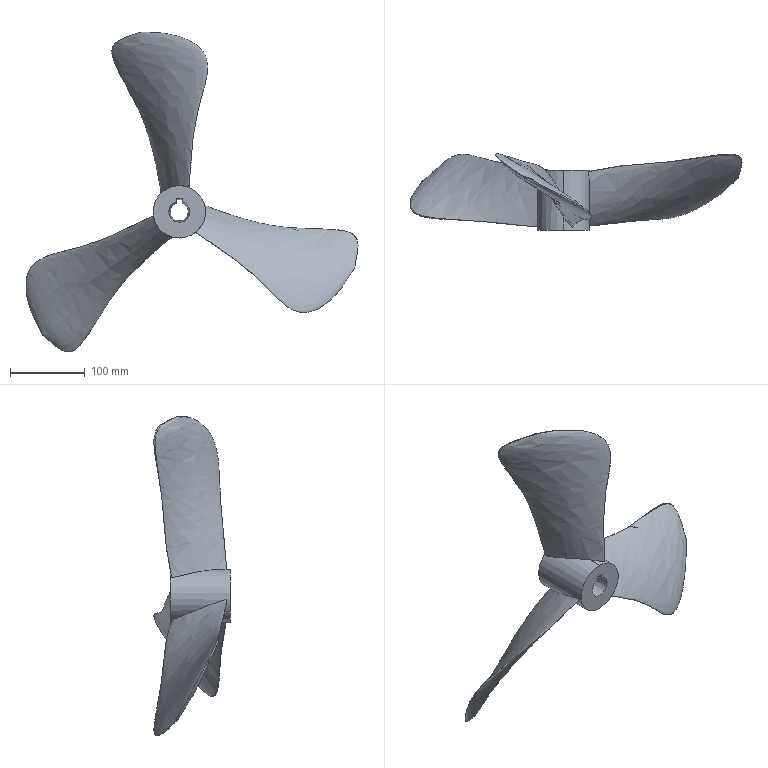Part | NX | features BREP 1 | 1 solid | 19 faces | box 443.196 x 101.773 x 427.156 mm | volume 901902 mm3 | plane 8 | spline 6 | cone 3 | cylinder 2 | commonest cylinder face diameters 70 x2